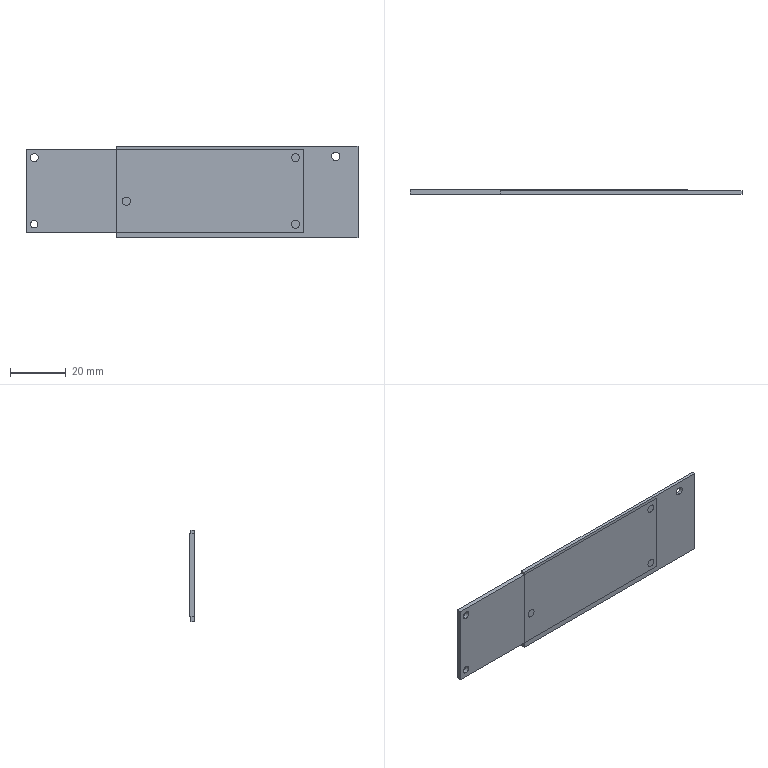Part | SolidWorks | features BaseBody 2 | 2 solids | 24 faces | box 119.5 x 1.6 x 33.1 mm | volume 8199 mm3 | cylinder 12 | plane 12 | commonest cylinder face diameters 3 x4 2.719 x2 2.825 x2 2.843 x2 2.882 x2
STEP:
#1=CARTESIAN_POINT('',(561.61,-1.6,-194.824));
#2=VERTEX_POINT('',#1);
#3=CARTESIAN_POINT('',(561.61,-1.6,-197.824));
#4=VERTEX_POINT('',#3);
#5=CARTESIAN_POINT('',(561.61,-1.6,-196.324));
#6=DIRECTION('',(0.,-1.,0.));
#7=DIRECTION('',(0.,0.,1.));
#8=AXIS2_PLACEMENT_3D('',#5,#6,#7);
#9=CIRCLE('',#8,1.5);
#10=EDGE_CURVE('',#2,#4,#9,.T.);
#11=ORIENTED_EDGE('',*,*,#10,.T.);
#12=CARTESIAN_POINT('',(561.61,-0.4,-197.824));
#13=VERTEX_POINT('',#12);
#14=CARTESIAN_POINT('',(561.61,-1.6,-197.824));
#15=DIRECTION('',(0.,1.,0.));
#16=VECTOR('',#15,1000.);
#17=LINE('',#14,#16);
#18=EDGE_CURVE('',#4,#13,#17,.T.);
#19=ORIENTED_EDGE('',*,*,#18,.T.);
#20=CARTESIAN_POINT('',(561.61,-0.4,-194.824));
#21=VERTEX_POINT('',#20);
#22=CARTESIAN_POINT('',(561.61,-0.4,-196.324));
#23=DIRECTION('',(0.,-1.,0.));
#24=DIRECTION('',(0.,0.,1.));
#25=AXIS2_PLACEMENT_3D('',#22,#23,#24);
#26=CIRCLE('',#25,1.5);
#27=EDGE_CURVE('',#21,#13,#26,.T.);
#28=ORIENTED_EDGE('',*,*,#27,.F.);
#29=CARTESIAN_POINT('',(561.61,-1.6,-194.824));
#30=DIRECTION('',(0.,1.,0.));
#31=VECTOR('',#30,1000.);
#32=LINE('',#29,#31);
#33=EDGE_CURVE('',#2,#21,#32,.T.);
#34=ORIENTED_EDGE('',*,*,#33,.F.);
#35=EDGE_LOOP('',(#11,#19,#28,#34));
#36=FACE_OUTER_BOUND('',#35,.T.);
#37=CARTESIAN_POINT('',(561.61,-1.6,-196.324));
#38=DIRECTION('',(0.,1.,0.));
#39=DIRECTION('',(0.,0.,1.));
#40=AXIS2_PLACEMENT_3D('',#37,#38,#39);
#41=CYLINDRICAL_SURFACE('',#40,1.5);
#42=ADVANCED_FACE('',(#36),#41,.F.);
#43=CARTESIAN_POINT('',(486.22,-1.6,-210.984));
#44=VERTEX_POINT('',#43);
#45=CARTESIAN_POINT('',(486.22,-1.6,-213.984));
#46=VERTEX_POINT('',#45);
#47=CARTESIAN_POINT('',(486.22,-1.6,-212.484));
#48=DIRECTION('',(0.,-1.,0.));
#49=DIRECTION('',(0.,0.,1.));
#50=AXIS2_PLACEMENT_3D('',#47,#48,#49);
#51=CIRCLE('',#50,1.5);
#52=EDGE_CURVE('',#44,#46,#51,.T.);
#53=ORIENTED_EDGE('',*,*,#52,.T.);
#54=CARTESIAN_POINT('',(486.22,-0.4,-213.984));
#55=VERTEX_POINT('',#54);
#56=CARTESIAN_POINT('',(486.22,-1.6,-213.984));
#57=DIRECTION('',(0.,1.,0.));
#58=VECTOR('',#57,1000.);
#59=LINE('',#56,#58);
#60=EDGE_CURVE('',#46,#55,#59,.T.);
#61=ORIENTED_EDGE('',*,*,#60,.T.);
#62=CARTESIAN_POINT('',(486.22,-0.4,-210.984));
#63=VERTEX_POINT('',#62);
#64=CARTESIAN_POINT('',(486.22,-0.4,-212.484));
#65=DIRECTION('',(0.,-1.,0.));
#66=DIRECTION('',(0.,0.,1.));
#67=AXIS2_PLACEMENT_3D('',#64,#65,#66);
#68=CIRCLE('',#67,1.5);
#69=EDGE_CURVE('',#63,#55,#68,.T.);
#70=ORIENTED_EDGE('',*,*,#69,.F.);
#71=CARTESIAN_POINT('',(486.22,-1.6,-210.984));
#72=DIRECTION('',(0.,1.,0.));
#73=VECTOR('',#72,1000.);
#74=LINE('',#71,#73);
#75=EDGE_CURVE('',#44,#63,#74,.T.);
#76=ORIENTED_EDGE('',*,*,#75,.F.);
#77=EDGE_LOOP('',(#53,#61,#70,#76));
#78=FACE_OUTER_BOUND('',#77,.T.);
#79=CARTESIAN_POINT('',(486.22,-1.6,-212.484));
#80=DIRECTION('',(0.,1.,0.));
#81=DIRECTION('',(0.,0.,1.));
#82=AXIS2_PLACEMENT_3D('',#79,#80,#81);
#83=CYLINDRICAL_SURFACE('',#82,1.5);
#84=ADVANCED_FACE('',(#78),#83,.F.);
#85=ORIENTED_EDGE('',*,*,#10,.F.);
#86=CARTESIAN_POINT('',(561.61,-1.6,-196.324));
#87=DIRECTION('',(0.,-1.,0.));
#88=DIRECTION('',(0.,0.,1.));
#89=AXIS2_PLACEMENT_3D('',#86,#87,#88);
#90=CIRCLE('',#89,1.5);
#91=EDGE_CURVE('',#4,#2,#90,.T.);
#92=ORIENTED_EDGE('',*,*,#91,.F.);
#93=EDGE_LOOP('',(#85,#92));
#94=FACE_BOUND('',#93,.T.);
#95=ORIENTED_EDGE('',*,*,#52,.F.);
#96=CARTESIAN_POINT('',(486.22,-1.6,-212.484));
#97=DIRECTION('',(0.,-1.,0.));
#98=DIRECTION('',(0.,0.,1.));
#99=AXIS2_PLACEMENT_3D('',#96,#97,#98);
#100=CIRCLE('',#99,1.5);
#101=EDGE_CURVE('',#46,#44,#100,.T.);
#102=ORIENTED_EDGE('',*,*,#101,.F.);
#103=EDGE_LOOP('',(#95,#102));
#104=FACE_BOUND('',#103,.T.);
#105=CARTESIAN_POINT('',(569.59,-1.6,-192.614));
#106=VERTEX_POINT('',#105);
#107=CARTESIAN_POINT('',(569.59,-1.6,-225.714));
#108=VERTEX_POINT('',#107);
#109=CARTESIAN_POINT('',(569.59,-1.6,-209.164));
#110=DIRECTION('',(0.,0.,-1.));
#111=VECTOR('',#110,1000.);
#112=LINE('',#109,#111);
#113=EDGE_CURVE('',#106,#108,#112,.T.);
#114=ORIENTED_EDGE('',*,*,#113,.F.);
#115=CARTESIAN_POINT('',(482.59,-1.6,-192.614));
#116=VERTEX_POINT('',#115);
#117=CARTESIAN_POINT('',(526.09,-1.6,-192.614));
#118=DIRECTION('',(1.,0.,0.));
#119=VECTOR('',#118,1000.);
#120=LINE('',#117,#119);
#121=EDGE_CURVE('',#116,#106,#120,.T.);
#122=ORIENTED_EDGE('',*,*,#121,.F.);
#123=CARTESIAN_POINT('',(482.59,-1.6,-225.714));
#124=VERTEX_POINT('',#123);
#125=CARTESIAN_POINT('',(482.59,-1.6,-209.164));
#126=DIRECTION('',(0.,0.,1.));
#127=VECTOR('',#126,1000.);
#128=LINE('',#125,#127);
#129=EDGE_CURVE('',#124,#116,#128,.T.);
#130=ORIENTED_EDGE('',*,*,#129,.F.);
#131=CARTESIAN_POINT('',(526.09,-1.6,-225.714));
#132=DIRECTION('',(-1.,0.,0.));
#133=VECTOR('',#132,1000.);
#134=LINE('',#131,#133);
#135=EDGE_CURVE('',#108,#124,#134,.T.);
#136=ORIENTED_EDGE('',*,*,#135,.F.);
#137=EDGE_LOOP('',(#114,#122,#130,#136));
#138=FACE_OUTER_BOUND('',#137,.T.);
#139=CARTESIAN_POINT('',(526.09,-1.6,-209.164));
#140=DIRECTION('',(0.,1.,0.));
#141=DIRECTION('',(0.,0.,1.));
#142=AXIS2_PLACEMENT_3D('',#139,#140,#141);
#143=PLANE('',#142);
#144=ADVANCED_FACE('',(#94,#104,#138),#143,.F.);
#145=ORIENTED_EDGE('',*,*,#18,.F.);
#146=ORIENTED_EDGE('',*,*,#91,.T.);
#147=ORIENTED_EDGE('',*,*,#33,.T.);
#148=CARTESIAN_POINT('',(561.61,-0.4,-196.324));
#149=DIRECTION('',(0.,-1.,0.));
#150=DIRECTION('',(0.,0.,1.));
#151=AXIS2_PLACEMENT_3D('',#148,#149,#150);
#152=CIRCLE('',#151,1.5);
#153=EDGE_CURVE('',#13,#21,#152,.T.);
#154=ORIENTED_EDGE('',*,*,#153,.F.);
#155=EDGE_LOOP('',(#145,#146,#147,#154));
#156=FACE_OUTER_BOUND('',#155,.T.);
#157=CARTESIAN_POINT('',(561.61,-1.6,-196.324));
#158=DIRECTION('',(0.,1.,0.));
#159=DIRECTION('',(0.,0.,1.));
#160=AXIS2_PLACEMENT_3D('',#157,#158,#159);
#161=CYLINDRICAL_SURFACE('',#160,1.5);
#162=ADVANCED_FACE('',(#156),#161,.F.);
#163=ORIENTED_EDGE('',*,*,#60,.F.);
#164=ORIENTED_EDGE('',*,*,#101,.T.);
#165=ORIENTED_EDGE('',*,*,#75,.T.);
#166=CARTESIAN_POINT('',(486.22,-0.4,-212.484));
#167=DIRECTION('',(0.,-1.,0.));
#168=DIRECTION('',(0.,0.,1.));
#169=AXIS2_PLACEMENT_3D('',#166,#167,#168);
#170=CIRCLE('',#169,1.5);
#171=EDGE_CURVE('',#55,#63,#170,.T.);
#172=ORIENTED_EDGE('',*,*,#171,.F.);
#173=EDGE_LOOP('',(#163,#164,#165,#172));
#174=FACE_OUTER_BOUND('',#173,.T.);
#175=CARTESIAN_POINT('',(486.22,-1.6,-212.484));
#176=DIRECTION('',(0.,1.,0.));
#177=DIRECTION('',(0.,0.,1.));
#178=AXIS2_PLACEMENT_3D('',#175,#176,#177);
#179=CYLINDRICAL_SURFACE('',#178,1.5);
#180=ADVANCED_FACE('',(#174),#179,.F.);
#181=CARTESIAN_POINT('',(569.59,-0.4,-225.714));
#182=VERTEX_POINT('',#181);
#183=CARTESIAN_POINT('',(569.59,-1.6,-225.714));
#184=DIRECTION('',(0.,-1.,0.));
#185=VECTOR('',#184,1000.);
#186=LINE('',#183,#185);
#187=EDGE_CURVE('',#182,#108,#186,.T.);
#188=ORIENTED_EDGE('',*,*,#187,.T.);
#189=ORIENTED_EDGE('',*,*,#135,.T.);
#190=CARTESIAN_POINT('',(482.59,-0.4,-225.714));
#191=VERTEX_POINT('',#190);
#192=CARTESIAN_POINT('',(482.59,-1.6,-225.714));
#193=DIRECTION('',(0.,1.,0.));
#194=VECTOR('',#193,1000.);
#195=LINE('',#192,#194);
#196=EDGE_CURVE('',#124,#191,#195,.T.);
#197=ORIENTED_EDGE('',*,*,#196,.T.);
#198=CARTESIAN_POINT('',(569.59,-0.4,-225.714));
#199=DIRECTION('',(1.,0.,0.));
#200=VECTOR('',#199,1000.);
#201=LINE('',#198,#200);
#202=EDGE_CURVE('',#191,#182,#201,.T.);
#203=ORIENTED_EDGE('',*,*,#202,.T.);
#204=EDGE_LOOP('',(#188,#189,#197,#203));
#205=FACE_OUTER_BOUND('',#204,.T.);
#206=CARTESIAN_POINT('',(569.59,-1.6,-225.714));
#207=DIRECTION('',(0.,0.,-1.));
#208=DIRECTION('',(-1.,0.,0.));
#209=AXIS2_PLACEMENT_3D('',#206,#207,#208);
#210=PLANE('',#209);
#211=ADVANCED_FACE('',(#205),#210,.T.);
#212=CARTESIAN_POINT('',(569.59,-0.4,-192.614));
#213=VERTEX_POINT('',#212);
#214=CARTESIAN_POINT('',(569.59,-1.6,-192.614));
#215=DIRECTION('',(0.,-1.,0.));
#216=VECTOR('',#215,1000.);
#217=LINE('',#214,#216);
#218=EDGE_CURVE('',#213,#106,#217,.T.);
#219=ORIENTED_EDGE('',*,*,#218,.T.);
#220=ORIENTED_EDGE('',*,*,#113,.T.);
#221=ORIENTED_EDGE('',*,*,#187,.F.);
#222=CARTESIAN_POINT('',(569.59,-0.4,-192.614));
#223=DIRECTION('',(0.,0.,1.));
#224=VECTOR('',#223,1000.);
#225=LINE('',#222,#224);
#226=EDGE_CURVE('',#182,#213,#225,.T.);
#227=ORIENTED_EDGE('',*,*,#226,.T.);
#228=EDGE_LOOP('',(#219,#220,#221,#227));
#229=FACE_OUTER_BOUND('',#228,.T.);
#230=CARTESIAN_POINT('',(569.59,-1.6,-192.614));
#231=DIRECTION('',(1.,0.,0.));
#232=DIRECTION('',(0.,0.,-1.));
#233=AXIS2_PLACEMENT_3D('',#230,#231,#232);
#234=PLANE('',#233);
#235=ADVANCED_FACE('',(#229),#234,.T.);
#236=CARTESIAN_POINT('',(482.59,-0.4,-192.614));
#237=VERTEX_POINT('',#236);
#238=CARTESIAN_POINT('',(482.59,-1.6,-192.614));
#239=DIRECTION('',(0.,-1.,0.));
#240=VECTOR('',#239,1000.);
#241=LINE('',#238,#240);
#242=EDGE_CURVE('',#237,#116,#241,.T.);
#243=ORIENTED_EDGE('',*,*,#242,.T.);
#244=ORIENTED_EDGE('',*,*,#121,.T.);
#245=ORIENTED_EDGE('',*,*,#218,.F.);
#246=CARTESIAN_POINT('',(482.59,-0.4,-192.614));
#247=DIRECTION('',(-1.,0.,0.));
#248=VECTOR('',#247,1000.);
#249=LINE('',#246,#248);
#250=EDGE_CURVE('',#213,#237,#249,.T.);
#251=ORIENTED_EDGE('',*,*,#250,.T.);
#252=EDGE_LOOP('',(#243,#244,#245,#251));
#253=FACE_OUTER_BOUND('',#252,.T.);
#254=CARTESIAN_POINT('',(482.59,-1.6,-192.614));
#255=DIRECTION('',(0.,0.,1.));
#256=DIRECTION('',(1.,0.,0.));
#257=AXIS2_PLACEMENT_3D('',#254,#255,#256);
#258=PLANE('',#257);
#259=ADVANCED_FACE('',(#253),#258,.T.);
#260=ORIENTED_EDGE('',*,*,#196,.F.);
#261=ORIENTED_EDGE('',*,*,#129,.T.);
#262=ORIENTED_EDGE('',*,*,#242,.F.);
#263=CARTESIAN_POINT('',(482.59,-0.4,-225.714));
#264=DIRECTION('',(0.,0.,-1.));
#265=VECTOR('',#264,1000.);
#266=LINE('',#263,#265);
#267=EDGE_CURVE('',#237,#191,#266,.T.);
#268=ORIENTED_EDGE('',*,*,#267,.T.);
#269=EDGE_LOOP('',(#260,#261,#262,#268));
#270=FACE_OUTER_BOUND('',#269,.T.);
#271=CARTESIAN_POINT('',(482.59,-1.6,-225.714));
#272=DIRECTION('',(-1.,0.,0.));
#273=DIRECTION('',(0.,0.,1.));
#274=AXIS2_PLACEMENT_3D('',#271,#272,#273);
#275=PLANE('',#274);
#276=ADVANCED_FACE('',(#270),#275,.T.);
#277=ORIENTED_EDGE('',*,*,#27,.T.);
#278=ORIENTED_EDGE('',*,*,#153,.T.);
#279=EDGE_LOOP('',(#277,#278));
#280=FACE_BOUND('',#279,.T.);
#281=ORIENTED_EDGE('',*,*,#69,.T.);
#282=ORIENTED_EDGE('',*,*,#171,.T.);
#283=EDGE_LOOP('',(#281,#282));
#284=FACE_BOUND('',#283,.T.);
#285=ORIENTED_EDGE('',*,*,#202,.F.);
#286=ORIENTED_EDGE('',*,*,#267,.F.);
#287=ORIENTED_EDGE('',*,*,#250,.F.);
#288=ORIENTED_EDGE('',*,*,#226,.F.);
#289=EDGE_LOOP('',(#285,#286,#287,#288));
#290=FACE_OUTER_BOUND('',#289,.T.);
#291=CARTESIAN_POINT('',(526.09,-0.4,-209.164));
#292=DIRECTION('',(0.,1.,0.));
#293=DIRECTION('',(0.,0.,1.));
#294=AXIS2_PLACEMENT_3D('',#291,#292,#293);
#295=PLANE('',#294);
#296=ADVANCED_FACE('',(#280,#284,#290),#295,.T.);
#297=CLOSED_SHELL('',(#42,#84,#144,#162,#180,#211,#235,#259,#276,#296));
#298=MANIFOLD_SOLID_BREP('',#297);
#299=CARTESIAN_POINT('',(547.081,-1.6,-198.186));
#300=VERTEX_POINT('',#299);
#301=CARTESIAN_POINT('',(547.081,-1.6,-195.362));
#302=VERTEX_POINT('',#301);
#303=CARTESIAN_POINT('',(547.081,-1.6,-196.774));
#304=DIRECTION('',(0.,1.,0.));
#305=DIRECTION('',(0.,0.,1.));
#306=AXIS2_PLACEMENT_3D('',#303,#304,#305);
#307=CIRCLE('',#306,1.412);
#308=EDGE_CURVE('',#300,#302,#307,.T.);
#309=ORIENTED_EDGE('',*,*,#308,.F.);
#310=CARTESIAN_POINT('',(547.081,0.,-198.186));
#311=VERTEX_POINT('',#310);
#312=CARTESIAN_POINT('',(547.081,0.,-198.186));
#313=DIRECTION('',(0.,1.,0.));
#314=VECTOR('',#313,1000.);
#315=LINE('',#312,#314);
#316=EDGE_CURVE('',#300,#311,#315,.T.);
#317=ORIENTED_EDGE('',*,*,#316,.T.);
#318=CARTESIAN_POINT('',(547.081,0.,-195.362));
#319=VERTEX_POINT('',#318);
#320=CARTESIAN_POINT('',(547.081,0.,-196.774));
#321=DIRECTION('',(0.,-1.,0.));
#322=DIRECTION('',(0.,0.,1.));
#323=AXIS2_PLACEMENT_3D('',#320,#321,#322);
#324=CIRCLE('',#323,1.412);
#325=EDGE_CURVE('',#319,#311,#324,.T.);
#326=ORIENTED_EDGE('',*,*,#325,.F.);
#327=CARTESIAN_POINT('',(547.081,0.,-195.362));
#328=DIRECTION('',(0.,1.,0.));
#329=VECTOR('',#328,1000.);
#330=LINE('',#327,#329);
#331=EDGE_CURVE('',#302,#319,#330,.T.);
#332=ORIENTED_EDGE('',*,*,#331,.F.);
#333=EDGE_LOOP('',(#309,#317,#326,#332));
#334=FACE_OUTER_BOUND('',#333,.T.);
#335=CARTESIAN_POINT('',(547.081,0.,-196.774));
#336=DIRECTION('',(0.,1.,0.));
#337=DIRECTION('',(0.,0.,1.));
#338=AXIS2_PLACEMENT_3D('',#335,#336,#337);
#339=CYLINDRICAL_SURFACE('',#338,1.412);
#340=ADVANCED_FACE('',(#334),#339,.F.);
#341=CARTESIAN_POINT('',(547.08,-1.6,-222.19));
#342=VERTEX_POINT('',#341);
#343=CARTESIAN_POINT('',(547.08,-1.6,-219.347));
#344=VERTEX_POINT('',#343);
#345=CARTESIAN_POINT('',(547.08,-1.6,-220.769));
#346=DIRECTION('',(0.,1.,0.));
#347=DIRECTION('',(0.,0.,1.));
#348=AXIS2_PLACEMENT_3D('',#345,#346,#347);
#349=CIRCLE('',#348,1.421);
#350=EDGE_CURVE('',#342,#344,#349,.T.);
#351=ORIENTED_EDGE('',*,*,#350,.F.);
#352=CARTESIAN_POINT('',(547.08,0.,-222.19));
#353=VERTEX_POINT('',#352);
#354=CARTESIAN_POINT('',(547.08,0.,-222.19));
#355=DIRECTION('',(0.,1.,0.));
#356=VECTOR('',#355,1000.);
#357=LINE('',#354,#356);
#358=EDGE_CURVE('',#342,#353,#357,.T.);
#359=ORIENTED_EDGE('',*,*,#358,.T.);
#360=CARTESIAN_POINT('',(547.08,0.,-219.347));
#361=VERTEX_POINT('',#360);
#362=CARTESIAN_POINT('',(547.08,0.,-220.769));
#363=DIRECTION('',(0.,-1.,0.));
#364=DIRECTION('',(0.,0.,1.));
#365=AXIS2_PLACEMENT_3D('',#362,#363,#364);
#366=CIRCLE('',#365,1.421);
#367=EDGE_CURVE('',#361,#353,#366,.T.);
#368=ORIENTED_EDGE('',*,*,#367,.F.);
#369=CARTESIAN_POINT('',(547.08,0.,-219.347));
#370=DIRECTION('',(0.,1.,0.));
#371=VECTOR('',#370,1000.);
#372=LINE('',#369,#371);
#373=EDGE_CURVE('',#344,#361,#372,.T.);
#374=ORIENTED_EDGE('',*,*,#373,.F.);
#375=EDGE_LOOP('',(#351,#359,#368,#374));
#376=FACE_OUTER_BOUND('',#375,.T.);
#377=CARTESIAN_POINT('',(547.08,0.,-220.769));
#378=DIRECTION('',(0.,1.,0.));
#379=DIRECTION('',(0.,0.,1.));
#380=AXIS2_PLACEMENT_3D('',#377,#378,#379);
#381=CYLINDRICAL_SURFACE('',#380,1.421);
#382=ADVANCED_FACE('',(#376),#381,.F.);
#383=CARTESIAN_POINT('',(453.068,-1.6,-198.213));
#384=VERTEX_POINT('',#383);
#385=CARTESIAN_POINT('',(453.068,-1.6,-195.33));
#386=VERTEX_POINT('',#385);
#387=CARTESIAN_POINT('',(453.068,-1.6,-196.772));
#388=DIRECTION('',(0.,1.,0.));
#389=DIRECTION('',(0.,0.,1.));
#390=AXIS2_PLACEMENT_3D('',#387,#388,#389);
#391=CIRCLE('',#390,1.441);
#392=EDGE_CURVE('',#384,#386,#391,.T.);
#393=ORIENTED_EDGE('',*,*,#392,.F.);
#394=CARTESIAN_POINT('',(453.068,0.,-198.213));
#395=VERTEX_POINT('',#394);
#396=CARTESIAN_POINT('',(453.068,0.,-198.213));
#397=DIRECTION('',(0.,1.,0.));
#398=VECTOR('',#397,1000.);
#399=LINE('',#396,#398);
#400=EDGE_CURVE('',#384,#395,#399,.T.);
#401=ORIENTED_EDGE('',*,*,#400,.T.);
#402=CARTESIAN_POINT('',(453.068,0.,-195.33));
#403=VERTEX_POINT('',#402);
#404=CARTESIAN_POINT('',(453.068,0.,-196.772));
#405=DIRECTION('',(0.,-1.,0.));
#406=DIRECTION('',(0.,0.,1.));
#407=AXIS2_PLACEMENT_3D('',#404,#405,#406);
#408=CIRCLE('',#407,1.441);
#409=EDGE_CURVE('',#403,#395,#408,.T.);
#410=ORIENTED_EDGE('',*,*,#409,.F.);
#411=CARTESIAN_POINT('',(453.068,0.,-195.33));
#412=DIRECTION('',(0.,1.,0.));
#413=VECTOR('',#412,1000.);
#414=LINE('',#411,#413);
#415=EDGE_CURVE('',#386,#403,#414,.T.);
#416=ORIENTED_EDGE('',*,*,#415,.F.);
#417=EDGE_LOOP('',(#393,#401,#410,#416));
#418=FACE_OUTER_BOUND('',#417,.T.);
#419=CARTESIAN_POINT('',(453.068,0.,-196.772));
#420=DIRECTION('',(0.,1.,0.));
#421=DIRECTION('',(0.,0.,1.));
#422=AXIS2_PLACEMENT_3D('',#419,#420,#421);
#423=CYLINDRICAL_SURFACE('',#422,1.441);
#424=ADVANCED_FACE('',(#418),#423,.F.);
#425=CARTESIAN_POINT('',(453.054,-1.6,-222.115));
#426=VERTEX_POINT('',#425);
#427=CARTESIAN_POINT('',(453.054,-1.6,-219.396));
#428=VERTEX_POINT('',#427);
#429=CARTESIAN_POINT('',(453.054,-1.6,-220.756));
#430=DIRECTION('',(0.,1.,0.));
#431=DIRECTION('',(0.,0.,1.));
#432=AXIS2_PLACEMENT_3D('',#429,#430,#431);
#433=CIRCLE('',#432,1.36);
#434=EDGE_CURVE('',#426,#428,#433,.T.);
#435=ORIENTED_EDGE('',*,*,#434,.F.);
#436=CARTESIAN_POINT('',(453.054,0.,-222.115));
#437=VERTEX_POINT('',#436);
#438=CARTESIAN_POINT('',(453.054,0.,-222.115));
#439=DIRECTION('',(0.,1.,0.));
#440=VECTOR('',#439,1000.);
#441=LINE('',#438,#440);
#442=EDGE_CURVE('',#426,#437,#441,.T.);
#443=ORIENTED_EDGE('',*,*,#442,.T.);
#444=CARTESIAN_POINT('',(453.054,0.,-219.396));
#445=VERTEX_POINT('',#444);
#446=CARTESIAN_POINT('',(453.054,0.,-220.756));
#447=DIRECTION('',(0.,-1.,0.));
#448=DIRECTION('',(0.,0.,1.));
#449=AXIS2_PLACEMENT_3D('',#446,#447,#448);
#450=CIRCLE('',#449,1.36);
#451=EDGE_CURVE('',#445,#437,#450,.T.);
#452=ORIENTED_EDGE('',*,*,#451,.F.);
#453=CARTESIAN_POINT('',(453.054,0.,-219.396));
#454=DIRECTION('',(0.,1.,0.));
#455=VECTOR('',#454,1000.);
#456=LINE('',#453,#455);
#457=EDGE_CURVE('',#428,#445,#456,.T.);
#458=ORIENTED_EDGE('',*,*,#457,.F.);
#459=EDGE_LOOP('',(#435,#443,#452,#458));
#460=FACE_OUTER_BOUND('',#459,.T.);
#461=CARTESIAN_POINT('',(453.054,0.,-220.756));
#462=DIRECTION('',(0.,1.,0.));
#463=DIRECTION('',(0.,0.,1.));
#464=AXIS2_PLACEMENT_3D('',#461,#462,#463);
#465=CYLINDRICAL_SURFACE('',#464,1.36);
#466=ADVANCED_FACE('',(#460),#465,.F.);
#467=ORIENTED_EDGE('',*,*,#325,.T.);
#468=CARTESIAN_POINT('',(547.081,0.,-196.774));
#469=DIRECTION('',(0.,-1.,0.));
#470=DIRECTION('',(0.,0.,1.));
#471=AXIS2_PLACEMENT_3D('',#468,#469,#470);
#472=CIRCLE('',#471,1.412);
#473=EDGE_CURVE('',#311,#319,#472,.T.);
#474=ORIENTED_EDGE('',*,*,#473,.T.);
#475=EDGE_LOOP('',(#467,#474));
#476=FACE_BOUND('',#475,.T.);
#477=ORIENTED_EDGE('',*,*,#367,.T.);
#478=CARTESIAN_POINT('',(547.08,0.,-220.769));
#479=DIRECTION('',(0.,-1.,0.));
#480=DIRECTION('',(0.,0.,1.));
#481=AXIS2_PLACEMENT_3D('',#478,#479,#480);
#482=CIRCLE('',#481,1.421);
#483=EDGE_CURVE('',#353,#361,#482,.T.);
#484=ORIENTED_EDGE('',*,*,#483,.T.);
#485=EDGE_LOOP('',(#477,#484));
#486=FACE_BOUND('',#485,.T.);
#487=ORIENTED_EDGE('',*,*,#409,.T.);
#488=CARTESIAN_POINT('',(453.068,0.,-196.772));
#489=DIRECTION('',(0.,-1.,0.));
#490=DIRECTION('',(0.,0.,1.));
#491=AXIS2_PLACEMENT_3D('',#488,#489,#490);
#492=CIRCLE('',#491,1.441);
#493=EDGE_CURVE('',#395,#403,#492,.T.);
#494=ORIENTED_EDGE('',*,*,#493,.T.);
#495=EDGE_LOOP('',(#487,#494));
#496=FACE_BOUND('',#495,.T.);
#497=ORIENTED_EDGE('',*,*,#451,.T.);
#498=CARTESIAN_POINT('',(453.054,0.,-220.756));
#499=DIRECTION('',(0.,-1.,0.));
#500=DIRECTION('',(0.,0.,1.));
#501=AXIS2_PLACEMENT_3D('',#498,#499,#500);
#502=CIRCLE('',#501,1.36);
#503=EDGE_CURVE('',#437,#445,#502,.T.);
#504=ORIENTED_EDGE('',*,*,#503,.T.);
#505=EDGE_LOOP('',(#497,#504));
#506=FACE_BOUND('',#505,.T.);
#507=CARTESIAN_POINT('',(450.09,0.,-223.764));
#508=VERTEX_POINT('',#507);
#509=CARTESIAN_POINT('',(450.09,0.,-193.764));
#510=VERTEX_POINT('',#509);
#511=CARTESIAN_POINT('',(450.09,0.,0.));
#512=DIRECTION('',(0.,0.,1.));
#513=VECTOR('',#512,1000.);
#514=LINE('',#511,#513);
#515=EDGE_CURVE('',#508,#510,#514,.T.);
#516=ORIENTED_EDGE('',*,*,#515,.T.);
#517=CARTESIAN_POINT('',(550.09,0.,-193.764));
#518=VERTEX_POINT('',#517);
#519=CARTESIAN_POINT('',(0.,0.,-193.764));
#520=DIRECTION('',(1.,0.,0.));
#521=VECTOR('',#520,1000.);
#522=LINE('',#519,#521);
#523=EDGE_CURVE('',#510,#518,#522,.T.);
#524=ORIENTED_EDGE('',*,*,#523,.T.);
#525=CARTESIAN_POINT('',(550.09,0.,-223.764));
#526=VERTEX_POINT('',#525);
#527=CARTESIAN_POINT('',(550.09,0.,0.));
#528=DIRECTION('',(0.,0.,-1.));
#529=VECTOR('',#528,1000.);
#530=LINE('',#527,#529);
#531=EDGE_CURVE('',#518,#526,#530,.T.);
#532=ORIENTED_EDGE('',*,*,#531,.T.);
#533=CARTESIAN_POINT('',(0.,0.,-223.764));
#534=DIRECTION('',(-1.,0.,0.));
#535=VECTOR('',#534,1000.);
#536=LINE('',#533,#535);
#537=EDGE_CURVE('',#526,#508,#536,.T.);
#538=ORIENTED_EDGE('',*,*,#537,.T.);
#539=EDGE_LOOP('',(#516,#524,#532,#538));
#540=FACE_OUTER_BOUND('',#539,.T.);
#541=CARTESIAN_POINT('',(0.,0.,0.));
#542=DIRECTION('',(0.,1.,0.));
#543=DIRECTION('',(0.,0.,1.));
#544=AXIS2_PLACEMENT_3D('',#541,#542,#543);
#545=PLANE('',#544);
#546=ADVANCED_FACE('',(#476,#486,#496,#506,#540),#545,.T.);
#547=ORIENTED_EDGE('',*,*,#316,.F.);
#548=CARTESIAN_POINT('',(547.081,-1.6,-196.774));
#549=DIRECTION('',(0.,1.,0.));
#550=DIRECTION('',(0.,0.,1.));
#551=AXIS2_PLACEMENT_3D('',#548,#549,#550);
#552=CIRCLE('',#551,1.412);
#553=EDGE_CURVE('',#302,#300,#552,.T.);
#554=ORIENTED_EDGE('',*,*,#553,.F.);
#555=ORIENTED_EDGE('',*,*,#331,.T.);
#556=ORIENTED_EDGE('',*,*,#473,.F.);
#557=EDGE_LOOP('',(#547,#554,#555,#556));
#558=FACE_OUTER_BOUND('',#557,.T.);
#559=CARTESIAN_POINT('',(547.081,0.,-196.774));
#560=DIRECTION('',(0.,1.,0.));
#561=DIRECTION('',(0.,0.,1.));
#562=AXIS2_PLACEMENT_3D('',#559,#560,#561);
#563=CYLINDRICAL_SURFACE('',#562,1.412);
#564=ADVANCED_FACE('',(#558),#563,.F.);
#565=ORIENTED_EDGE('',*,*,#358,.F.);
#566=CARTESIAN_POINT('',(547.08,-1.6,-220.769));
#567=DIRECTION('',(0.,1.,0.));
#568=DIRECTION('',(0.,0.,1.));
#569=AXIS2_PLACEMENT_3D('',#566,#567,#568);
#570=CIRCLE('',#569,1.421);
#571=EDGE_CURVE('',#344,#342,#570,.T.);
#572=ORIENTED_EDGE('',*,*,#571,.F.);
#573=ORIENTED_EDGE('',*,*,#373,.T.);
#574=ORIENTED_EDGE('',*,*,#483,.F.);
#575=EDGE_LOOP('',(#565,#572,#573,#574));
#576=FACE_OUTER_BOUND('',#575,.T.);
#577=CARTESIAN_POINT('',(547.08,0.,-220.769));
#578=DIRECTION('',(0.,1.,0.));
#579=DIRECTION('',(0.,0.,1.));
#580=AXIS2_PLACEMENT_3D('',#577,#578,#579);
#581=CYLINDRICAL_SURFACE('',#580,1.421);
#582=ADVANCED_FACE('',(#576),#581,.F.);
#583=ORIENTED_EDGE('',*,*,#400,.F.);
#584=CARTESIAN_POINT('',(453.068,-1.6,-196.772));
#585=DIRECTION('',(0.,1.,0.));
#586=DIRECTION('',(0.,0.,1.));
#587=AXIS2_PLACEMENT_3D('',#584,#585,#586);
#588=CIRCLE('',#587,1.441);
#589=EDGE_CURVE('',#386,#384,#588,.T.);
#590=ORIENTED_EDGE('',*,*,#589,.F.);
#591=ORIENTED_EDGE('',*,*,#415,.T.);
#592=ORIENTED_EDGE('',*,*,#493,.F.);
#593=EDGE_LOOP('',(#583,#590,#591,#592));
#594=FACE_OUTER_BOUND('',#593,.T.);
#595=CARTESIAN_POINT('',(453.068,0.,-196.772));
#596=DIRECTION('',(0.,1.,0.));
#597=DIRECTION('',(0.,0.,1.));
#598=AXIS2_PLACEMENT_3D('',#595,#596,#597);
#599=CYLINDRICAL_SURFACE('',#598,1.441);
#600=ADVANCED_FACE('',(#594),#599,.F.);
#601=ORIENTED_EDGE('',*,*,#442,.F.);
#602=CARTESIAN_POINT('',(453.054,-1.6,-220.756));
#603=DIRECTION('',(0.,1.,0.));
#604=DIRECTION('',(0.,0.,1.));
#605=AXIS2_PLACEMENT_3D('',#602,#603,#604);
#606=CIRCLE('',#605,1.36);
#607=EDGE_CURVE('',#428,#426,#606,.T.);
#608=ORIENTED_EDGE('',*,*,#607,.F.);
#609=ORIENTED_EDGE('',*,*,#457,.T.);
#610=ORIENTED_EDGE('',*,*,#503,.F.);
#611=EDGE_LOOP('',(#601,#608,#609,#610));
#612=FACE_OUTER_BOUND('',#611,.T.);
#613=CARTESIAN_POINT('',(453.054,0.,-220.756));
#614=DIRECTION('',(0.,1.,0.));
#615=DIRECTION('',(0.,0.,1.));
#616=AXIS2_PLACEMENT_3D('',#613,#614,#615);
#617=CYLINDRICAL_SURFACE('',#616,1.36);
#618=ADVANCED_FACE('',(#612),#617,.F.);
#619=CARTESIAN_POINT('',(550.09,-1.6,-193.764));
#620=VERTEX_POINT('',#619);
#621=CARTESIAN_POINT('',(550.09,0.,-193.764));
#622=DIRECTION('',(0.,1.,0.));
#623=VECTOR('',#622,1000.);
#624=LINE('',#621,#623);
#625=EDGE_CURVE('',#620,#518,#624,.T.);
#626=ORIENTED_EDGE('',*,*,#625,.T.);
#627=ORIENTED_EDGE('',*,*,#523,.F.);
#628=CARTESIAN_POINT('',(450.09,-1.6,-193.764));
#629=VERTEX_POINT('',#628);
#630=CARTESIAN_POINT('',(450.09,0.,-193.764));
#631=DIRECTION('',(0.,-1.,0.));
#632=VECTOR('',#631,1000.);
#633=LINE('',#630,#632);
#634=EDGE_CURVE('',#510,#629,#633,.T.);
#635=ORIENTED_EDGE('',*,*,#634,.T.);
#636=CARTESIAN_POINT('',(450.09,-1.6,-193.764));
#637=DIRECTION('',(1.,0.,0.));
#638=VECTOR('',#637,1000.);
#639=LINE('',#636,#638);
#640=EDGE_CURVE('',#629,#620,#639,.T.);
#641=ORIENTED_EDGE('',*,*,#640,.T.);
#642=EDGE_LOOP('',(#626,#627,#635,#641));
#643=FACE_OUTER_BOUND('',#642,.T.);
#644=CARTESIAN_POINT('',(450.09,0.,-193.764));
#645=DIRECTION('',(0.,0.,1.));
#646=DIRECTION('',(1.,0.,0.));
#647=AXIS2_PLACEMENT_3D('',#644,#645,#646);
#648=PLANE('',#647);
#649=ADVANCED_FACE('',(#643),#648,.T.);
#650=ORIENTED_EDGE('',*,*,#634,.F.);
#651=ORIENTED_EDGE('',*,*,#515,.F.);
#652=CARTESIAN_POINT('',(450.09,-1.6,-223.764));
#653=VERTEX_POINT('',#652);
#654=CARTESIAN_POINT('',(450.09,0.,-223.764));
#655=DIRECTION('',(0.,-1.,0.));
#656=VECTOR('',#655,1000.);
#657=LINE('',#654,#656);
#658=EDGE_CURVE('',#508,#653,#657,.T.);
#659=ORIENTED_EDGE('',*,*,#658,.T.);
#660=CARTESIAN_POINT('',(450.09,-1.6,-223.764));
#661=DIRECTION('',(0.,0.,1.));
#662=VECTOR('',#661,1000.);
#663=LINE('',#660,#662);
#664=EDGE_CURVE('',#653,#629,#663,.T.);
#665=ORIENTED_EDGE('',*,*,#664,.T.);
#666=EDGE_LOOP('',(#650,#651,#659,#665));
#667=FACE_OUTER_BOUND('',#666,.T.);
#668=CARTESIAN_POINT('',(450.09,0.,-223.764));
#669=DIRECTION('',(-1.,0.,0.));
#670=DIRECTION('',(0.,0.,1.));
#671=AXIS2_PLACEMENT_3D('',#668,#669,#670);
#672=PLANE('',#671);
#673=ADVANCED_FACE('',(#667),#672,.T.);
#674=ORIENTED_EDGE('',*,*,#658,.F.);
#675=ORIENTED_EDGE('',*,*,#537,.F.);
#676=CARTESIAN_POINT('',(550.09,-1.6,-223.764));
#677=VERTEX_POINT('',#676);
#678=CARTESIAN_POINT('',(550.09,0.,-223.764));
#679=DIRECTION('',(0.,-1.,0.));
#680=VECTOR('',#679,1000.);
#681=LINE('',#678,#680);
#682=EDGE_CURVE('',#526,#677,#681,.T.);
#683=ORIENTED_EDGE('',*,*,#682,.T.);
#684=CARTESIAN_POINT('',(550.09,-1.6,-223.764));
#685=DIRECTION('',(-1.,0.,0.));
#686=VECTOR('',#685,1000.);
#687=LINE('',#684,#686);
#688=EDGE_CURVE('',#677,#653,#687,.T.);
#689=ORIENTED_EDGE('',*,*,#688,.T.);
#690=EDGE_LOOP('',(#674,#675,#683,#689));
#691=FACE_OUTER_BOUND('',#690,.T.);
#692=CARTESIAN_POINT('',(550.09,0.,-223.764));
#693=DIRECTION('',(0.,0.,-1.));
#694=DIRECTION('',(-1.,0.,0.));
#695=AXIS2_PLACEMENT_3D('',#692,#693,#694);
#696=PLANE('',#695);
#697=ADVANCED_FACE('',(#691),#696,.T.);
#698=ORIENTED_EDGE('',*,*,#682,.F.);
#699=ORIENTED_EDGE('',*,*,#531,.F.);
#700=ORIENTED_EDGE('',*,*,#625,.F.);
#701=CARTESIAN_POINT('',(550.09,-1.6,-193.764));
#702=DIRECTION('',(0.,0.,-1.));
#703=VECTOR('',#702,1000.);
#704=LINE('',#701,#703);
#705=EDGE_CURVE('',#620,#677,#704,.T.);
#706=ORIENTED_EDGE('',*,*,#705,.T.);
#707=EDGE_LOOP('',(#698,#699,#700,#706));
#708=FACE_OUTER_BOUND('',#707,.T.);
#709=CARTESIAN_POINT('',(550.09,0.,-193.764));
#710=DIRECTION('',(1.,0.,0.));
#711=DIRECTION('',(0.,0.,-1.));
#712=AXIS2_PLACEMENT_3D('',#709,#710,#711);
#713=PLANE('',#712);
#714=ADVANCED_FACE('',(#708),#713,.T.);
#715=ORIENTED_EDGE('',*,*,#553,.T.);
#716=ORIENTED_EDGE('',*,*,#308,.T.);
#717=EDGE_LOOP('',(#715,#716));
#718=FACE_BOUND('',#717,.T.);
#719=ORIENTED_EDGE('',*,*,#571,.T.);
#720=ORIENTED_EDGE('',*,*,#350,.T.);
#721=EDGE_LOOP('',(#719,#720));
#722=FACE_BOUND('',#721,.T.);
#723=ORIENTED_EDGE('',*,*,#589,.T.);
#724=ORIENTED_EDGE('',*,*,#392,.T.);
#725=EDGE_LOOP('',(#723,#724));
#726=FACE_BOUND('',#725,.T.);
#727=ORIENTED_EDGE('',*,*,#607,.T.);
#728=ORIENTED_EDGE('',*,*,#434,.T.);
#729=EDGE_LOOP('',(#727,#728));
#730=FACE_BOUND('',#729,.T.);
#731=ORIENTED_EDGE('',*,*,#688,.F.);
#732=ORIENTED_EDGE('',*,*,#705,.F.);
#733=ORIENTED_EDGE('',*,*,#640,.F.);
#734=ORIENTED_EDGE('',*,*,#664,.F.);
#735=EDGE_LOOP('',(#731,#732,#733,#734));
#736=FACE_OUTER_BOUND('',#735,.T.);
#737=CARTESIAN_POINT('',(0.,-1.6,0.));
#738=DIRECTION('',(0.,1.,0.));
#739=DIRECTION('',(0.,0.,1.));
#740=AXIS2_PLACEMENT_3D('',#737,#738,#739);
#741=PLANE('',#740);
#742=ADVANCED_FACE('',(#718,#722,#726,#730,#736),#741,.F.);
#743=CLOSED_SHELL('',(#340,#382,#424,#466,#546,#564,#582,#600,#618,#649,#673,#697,#714,#742));
#744=MANIFOLD_SOLID_BREP('',#743);
#745=CARTESIAN_POINT('',(0.,0.,0.));
#746=DIRECTION('',(0.,0.,1.));
#747=DIRECTION('',(1.,0.,0.));
#748=AXIS2_PLACEMENT_3D('',#745,#746,#747);
#749=(LENGTH_UNIT()NAMED_UNIT(*)SI_UNIT(.MILLI.,.METRE.));
#750=UNCERTAINTY_MEASURE_WITH_UNIT(LENGTH_MEASURE(0.00001),#749,'','');
#751=(NAMED_UNIT(*)PLANE_ANGLE_UNIT()SI_UNIT($,.RADIAN.));
#752=(NAMED_UNIT(*)SI_UNIT($,.STERADIAN.)SOLID_ANGLE_UNIT());
#753=(GEOMETRIC_REPRESENTATION_CONTEXT(3)GLOBAL_UNCERTAINTY_ASSIGNED_CONTEXT((#750))GLOBAL_UNIT_ASSIGNED_CONTEXT((#749,#751,#752))REPRESENTATION_CONTEXT('',''));
#754=ADVANCED_BREP_SHAPE_REPRESENTATION('',(#298,#744,#748),#753);